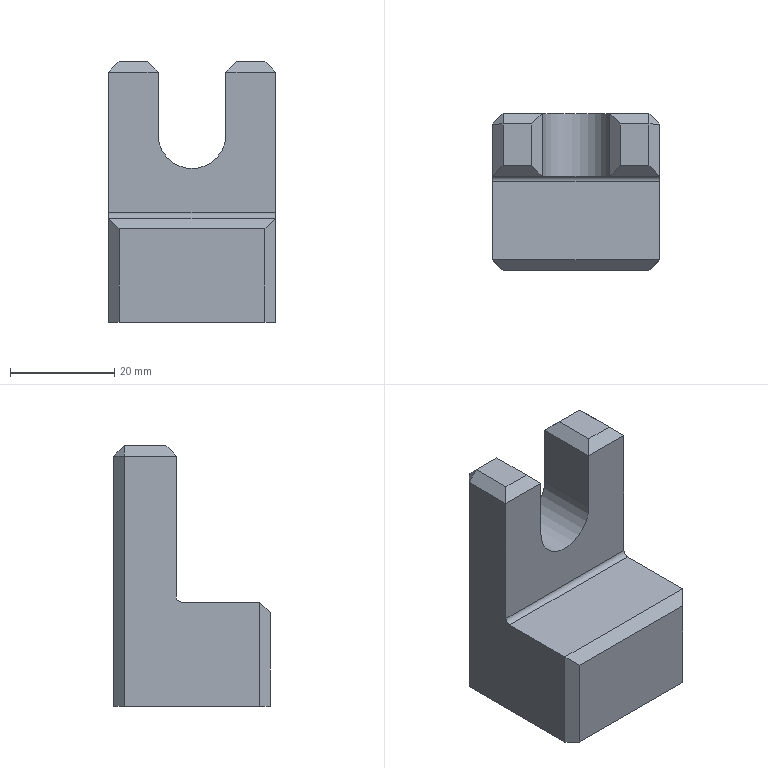Part | NX | features solid 2 | 1 solid | 30 faces | box 32 x 30 x 50 mm | volume 27056 mm3 | plane 26 | cylinder 3 | cone 1 | commonest cylinder face diameters 2 x1 5 x1 13 x1
STEP:
#1=CARTESIAN_POINT('',(8.5,703.,-103.));
#2=VERTEX_POINT('',#1);
#3=CARTESIAN_POINT('',(8.5,695.,-103.));
#4=VERTEX_POINT('',#3);
#5=CARTESIAN_POINT('',(8.5,693.,-103.));
#6=DIRECTION('',(0.,-1.,0.));
#7=VECTOR('',#6,1000.);
#8=LINE('',#5,#7);
#9=EDGE_CURVE('',#2,#4,#8,.T.);
#10=ORIENTED_EDGE('',*,*,#9,.T.);
#11=CARTESIAN_POINT('',(14.,695.,-103.));
#12=VERTEX_POINT('',#11);
#13=CARTESIAN_POINT('',(-16.,695.,-103.));
#14=DIRECTION('',(1.,0.,0.));
#15=VECTOR('',#14,1000.);
#16=LINE('',#13,#15);
#17=EDGE_CURVE('',#4,#12,#16,.T.);
#18=ORIENTED_EDGE('',*,*,#17,.T.);
#19=CARTESIAN_POINT('',(14.,703.,-103.));
#20=VERTEX_POINT('',#19);
#21=CARTESIAN_POINT('',(14.,705.,-103.));
#22=DIRECTION('',(0.,1.,0.));
#23=VECTOR('',#22,1000.);
#24=LINE('',#21,#23);
#25=EDGE_CURVE('',#12,#20,#24,.T.);
#26=ORIENTED_EDGE('',*,*,#25,.T.);
#27=CARTESIAN_POINT('',(6.5,703.,-103.));
#28=DIRECTION('',(-1.,0.,0.));
#29=VECTOR('',#28,1000.);
#30=LINE('',#27,#29);
#31=EDGE_CURVE('',#20,#2,#30,.T.);
#32=ORIENTED_EDGE('',*,*,#31,.T.);
#33=EDGE_LOOP('',(#10,#18,#26,#32));
#34=FACE_BOUND('',#33,.T.);
#35=CARTESIAN_POINT('',(-16.,693.,-103.));
#36=DIRECTION('',(0.,0.,1.));
#37=DIRECTION('',(-1.,0.,0.));
#38=AXIS2_PLACEMENT_3D('',#35,#36,#37);
#39=PLANE('',#38);
#40=ADVANCED_FACE('',(#34),#39,.T.);
#41=CARTESIAN_POINT('',(16.,703.,-153.));
#42=VERTEX_POINT('',#41);
#43=CARTESIAN_POINT('',(16.,703.,-105.));
#44=VERTEX_POINT('',#43);
#45=CARTESIAN_POINT('',(16.,703.,-133.));
#46=DIRECTION('',(0.,0.,1.));
#47=VECTOR('',#46,1000.);
#48=LINE('',#45,#47);
#49=EDGE_CURVE('',#42,#44,#48,.T.);
#50=ORIENTED_EDGE('',*,*,#49,.T.);
#51=CARTESIAN_POINT('',(16.,693.,-105.));
#52=VERTEX_POINT('',#51);
#53=CARTESIAN_POINT('',(16.,693.,-105.));
#54=DIRECTION('',(0.,-1.,0.));
#55=VECTOR('',#54,1000.);
#56=LINE('',#53,#55);
#57=EDGE_CURVE('',#44,#52,#56,.T.);
#58=ORIENTED_EDGE('',*,*,#57,.T.);
#59=CARTESIAN_POINT('',(16.,693.,-132.));
#60=VERTEX_POINT('',#59);
#61=CARTESIAN_POINT('',(16.,693.,-103.));
#62=DIRECTION('',(0.,0.,1.));
#63=VECTOR('',#62,1000.);
#64=LINE('',#61,#63);
#65=EDGE_CURVE('',#60,#52,#64,.T.);
#66=ORIENTED_EDGE('',*,*,#65,.F.);
#67=CARTESIAN_POINT('',(16.,692.,-133.));
#68=VERTEX_POINT('',#67);
#69=CARTESIAN_POINT('',(16.,692.,-132.));
#70=DIRECTION('',(-1.,0.,0.));
#71=DIRECTION('',(0.,0.,-1.));
#72=AXIS2_PLACEMENT_3D('',#69,#70,#71);
#73=CIRCLE('',#72,1.);
#74=EDGE_CURVE('',#60,#68,#73,.T.);
#75=ORIENTED_EDGE('',*,*,#74,.T.);
#76=CARTESIAN_POINT('',(16.,677.,-133.));
#77=VERTEX_POINT('',#76);
#78=CARTESIAN_POINT('',(16.,675.,-133.));
#79=DIRECTION('',(0.,1.,0.));
#80=VECTOR('',#79,1000.);
#81=LINE('',#78,#80);
#82=EDGE_CURVE('',#77,#68,#81,.T.);
#83=ORIENTED_EDGE('',*,*,#82,.F.);
#84=CARTESIAN_POINT('',(16.,677.,-153.));
#85=VERTEX_POINT('',#84);
#86=CARTESIAN_POINT('',(16.,677.,-153.));
#87=DIRECTION('',(0.,0.,-1.));
#88=VECTOR('',#87,1000.);
#89=LINE('',#86,#88);
#90=EDGE_CURVE('',#77,#85,#89,.T.);
#91=ORIENTED_EDGE('',*,*,#90,.T.);
#92=CARTESIAN_POINT('',(16.,675.,-153.));
#93=DIRECTION('',(0.,1.,0.));
#94=VECTOR('',#93,1000.);
#95=LINE('',#92,#94);
#96=EDGE_CURVE('',#85,#42,#95,.T.);
#97=ORIENTED_EDGE('',*,*,#96,.T.);
#98=EDGE_LOOP('',(#50,#58,#66,#75,#83,#91,#97));
#99=FACE_BOUND('',#98,.T.);
#100=CARTESIAN_POINT('',(16.,675.,-133.));
#101=DIRECTION('',(-1.,0.,0.));
#102=DIRECTION('',(0.,0.,-1.));
#103=AXIS2_PLACEMENT_3D('',#100,#101,#102);
#104=PLANE('',#103);
#105=ADVANCED_FACE('',(#99),#104,.F.);
#106=CARTESIAN_POINT('',(0.,705.,-145.5));
#107=VERTEX_POINT('',#106);
#108=CARTESIAN_POINT('',(0.,705.,-143.));
#109=DIRECTION('',(0.,-1.,0.));
#110=DIRECTION('',(0.,0.,-1.));
#111=AXIS2_PLACEMENT_3D('',#108,#109,#110);
#112=CIRCLE('',#111,2.5);
#113=EDGE_CURVE('',#107,#107,#112,.T.);
#114=ORIENTED_EDGE('',*,*,#113,.T.);
#115=EDGE_LOOP('',(#114));
#116=FACE_BOUND('',#115,.T.);
#117=CARTESIAN_POINT('',(6.5,705.,-117.));
#118=VERTEX_POINT('',#117);
#119=CARTESIAN_POINT('',(6.5,705.,-105.));
#120=VERTEX_POINT('',#119);
#121=CARTESIAN_POINT('',(6.5,705.,-103.));
#122=DIRECTION('',(0.,0.,1.));
#123=VECTOR('',#122,1000.);
#124=LINE('',#121,#123);
#125=EDGE_CURVE('',#118,#120,#124,.T.);
#126=ORIENTED_EDGE('',*,*,#125,.T.);
#127=CARTESIAN_POINT('',(14.,705.,-105.));
#128=VERTEX_POINT('',#127);
#129=CARTESIAN_POINT('',(16.,705.,-105.));
#130=DIRECTION('',(1.,0.,0.));
#131=VECTOR('',#130,1000.);
#132=LINE('',#129,#131);
#133=EDGE_CURVE('',#120,#128,#132,.T.);
#134=ORIENTED_EDGE('',*,*,#133,.T.);
#135=CARTESIAN_POINT('',(14.,705.,-153.));
#136=VERTEX_POINT('',#135);
#137=CARTESIAN_POINT('',(14.,705.,-133.));
#138=DIRECTION('',(0.,0.,-1.));
#139=VECTOR('',#138,1000.);
#140=LINE('',#137,#139);
#141=EDGE_CURVE('',#128,#136,#140,.T.);
#142=ORIENTED_EDGE('',*,*,#141,.T.);
#143=CARTESIAN_POINT('',(-14.,705.,-153.));
#144=VERTEX_POINT('',#143);
#145=CARTESIAN_POINT('',(16.,705.,-153.));
#146=DIRECTION('',(-1.,0.,0.));
#147=VECTOR('',#146,1000.);
#148=LINE('',#145,#147);
#149=EDGE_CURVE('',#136,#144,#148,.T.);
#150=ORIENTED_EDGE('',*,*,#149,.T.);
#151=CARTESIAN_POINT('',(-14.,705.,-105.));
#152=VERTEX_POINT('',#151);
#153=CARTESIAN_POINT('',(-14.,705.,-103.));
#154=DIRECTION('',(0.,0.,1.));
#155=VECTOR('',#154,1000.);
#156=LINE('',#153,#155);
#157=EDGE_CURVE('',#144,#152,#156,.T.);
#158=ORIENTED_EDGE('',*,*,#157,.T.);
#159=CARTESIAN_POINT('',(-6.5,705.,-105.));
#160=VERTEX_POINT('',#159);
#161=CARTESIAN_POINT('',(-6.5,705.,-105.));
#162=DIRECTION('',(1.,0.,0.));
#163=VECTOR('',#162,1000.);
#164=LINE('',#161,#163);
#165=EDGE_CURVE('',#152,#160,#164,.T.);
#166=ORIENTED_EDGE('',*,*,#165,.T.);
#167=CARTESIAN_POINT('',(-6.5,705.,-117.));
#168=VERTEX_POINT('',#167);
#169=CARTESIAN_POINT('',(-6.5,705.,-103.));
#170=DIRECTION('',(0.,0.,1.));
#171=VECTOR('',#170,1000.);
#172=LINE('',#169,#171);
#173=EDGE_CURVE('',#168,#160,#172,.T.);
#174=ORIENTED_EDGE('',*,*,#173,.F.);
#175=CARTESIAN_POINT('',(0.,705.,-117.));
#176=DIRECTION('',(0.,1.,0.));
#177=DIRECTION('',(0.,0.,1.));
#178=AXIS2_PLACEMENT_3D('',#175,#176,#177);
#179=CIRCLE('',#178,6.5);
#180=EDGE_CURVE('',#118,#168,#179,.T.);
#181=ORIENTED_EDGE('',*,*,#180,.F.);
#182=EDGE_LOOP('',(#126,#134,#142,#150,#158,#166,#174,#181));
#183=FACE_BOUND('',#182,.T.);
#184=CARTESIAN_POINT('',(16.,705.,-133.));
#185=DIRECTION('',(0.,-1.,0.));
#186=DIRECTION('',(0.,0.,-1.));
#187=AXIS2_PLACEMENT_3D('',#184,#185,#186);
#188=PLANE('',#187);
#189=ADVANCED_FACE('',(#116,#183),#188,.F.);
#190=CARTESIAN_POINT('',(-16.,677.,-133.));
#191=VERTEX_POINT('',#190);
#192=CARTESIAN_POINT('',(-16.,692.,-133.));
#193=VERTEX_POINT('',#192);
#194=CARTESIAN_POINT('',(-16.,675.,-133.));
#195=DIRECTION('',(0.,1.,0.));
#196=VECTOR('',#195,1000.);
#197=LINE('',#194,#196);
#198=EDGE_CURVE('',#191,#193,#197,.T.);
#199=ORIENTED_EDGE('',*,*,#198,.T.);
#200=CARTESIAN_POINT('',(-16.,693.,-132.));
#201=VERTEX_POINT('',#200);
#202=CARTESIAN_POINT('',(-16.,692.,-132.));
#203=DIRECTION('',(-1.,0.,0.));
#204=DIRECTION('',(0.,0.,-1.));
#205=AXIS2_PLACEMENT_3D('',#202,#203,#204);
#206=CIRCLE('',#205,1.);
#207=EDGE_CURVE('',#193,#201,#206,.F.);
#208=ORIENTED_EDGE('',*,*,#207,.T.);
#209=CARTESIAN_POINT('',(-16.,693.,-105.));
#210=VERTEX_POINT('',#209);
#211=CARTESIAN_POINT('',(-16.,693.,-103.));
#212=DIRECTION('',(0.,0.,1.));
#213=VECTOR('',#212,1000.);
#214=LINE('',#211,#213);
#215=EDGE_CURVE('',#201,#210,#214,.T.);
#216=ORIENTED_EDGE('',*,*,#215,.T.);
#217=CARTESIAN_POINT('',(-16.,703.,-105.));
#218=VERTEX_POINT('',#217);
#219=CARTESIAN_POINT('',(-16.,675.,-105.));
#220=DIRECTION('',(0.,1.,0.));
#221=VECTOR('',#220,1000.);
#222=LINE('',#219,#221);
#223=EDGE_CURVE('',#210,#218,#222,.T.);
#224=ORIENTED_EDGE('',*,*,#223,.T.);
#225=CARTESIAN_POINT('',(-16.,703.,-153.));
#226=VERTEX_POINT('',#225);
#227=CARTESIAN_POINT('',(-16.,703.,-153.));
#228=DIRECTION('',(0.,0.,-1.));
#229=VECTOR('',#228,1000.);
#230=LINE('',#227,#229);
#231=EDGE_CURVE('',#218,#226,#230,.T.);
#232=ORIENTED_EDGE('',*,*,#231,.T.);
#233=CARTESIAN_POINT('',(-16.,677.,-153.));
#234=VERTEX_POINT('',#233);
#235=CARTESIAN_POINT('',(-16.,675.,-153.));
#236=DIRECTION('',(0.,1.,0.));
#237=VECTOR('',#236,1000.);
#238=LINE('',#235,#237);
#239=EDGE_CURVE('',#234,#226,#238,.T.);
#240=ORIENTED_EDGE('',*,*,#239,.F.);
#241=CARTESIAN_POINT('',(-16.,677.,-133.));
#242=DIRECTION('',(0.,0.,1.));
#243=VECTOR('',#242,1000.);
#244=LINE('',#241,#243);
#245=EDGE_CURVE('',#234,#191,#244,.T.);
#246=ORIENTED_EDGE('',*,*,#245,.T.);
#247=EDGE_LOOP('',(#199,#208,#216,#224,#232,#240,#246));
#248=FACE_BOUND('',#247,.T.);
#249=CARTESIAN_POINT('',(-16.,675.,-133.));
#250=DIRECTION('',(-1.,0.,0.));
#251=DIRECTION('',(0.,0.,-1.));
#252=AXIS2_PLACEMENT_3D('',#249,#250,#251);
#253=PLANE('',#252);
#254=ADVANCED_FACE('',(#248),#253,.T.);
#255=CARTESIAN_POINT('',(14.,675.,-153.));
#256=VERTEX_POINT('',#255);
#257=CARTESIAN_POINT('',(-14.,675.,-153.));
#258=VERTEX_POINT('',#257);
#259=CARTESIAN_POINT('',(16.,675.,-153.));
#260=DIRECTION('',(-1.,0.,0.));
#261=VECTOR('',#260,1000.);
#262=LINE('',#259,#261);
#263=EDGE_CURVE('',#256,#258,#262,.T.);
#264=ORIENTED_EDGE('',*,*,#263,.F.);
#265=CARTESIAN_POINT('',(14.,675.,-135.));
#266=VERTEX_POINT('',#265);
#267=CARTESIAN_POINT('',(14.,675.,-133.));
#268=DIRECTION('',(0.,0.,1.));
#269=VECTOR('',#268,1000.);
#270=LINE('',#267,#269);
#271=EDGE_CURVE('',#256,#266,#270,.T.);
#272=ORIENTED_EDGE('',*,*,#271,.T.);
#273=CARTESIAN_POINT('',(-14.,675.,-135.));
#274=VERTEX_POINT('',#273);
#275=CARTESIAN_POINT('',(16.,675.,-135.));
#276=DIRECTION('',(-1.,0.,0.));
#277=VECTOR('',#276,1000.);
#278=LINE('',#275,#277);
#279=EDGE_CURVE('',#266,#274,#278,.T.);
#280=ORIENTED_EDGE('',*,*,#279,.T.);
#281=CARTESIAN_POINT('',(-14.,675.,-133.));
#282=DIRECTION('',(0.,0.,-1.));
#283=VECTOR('',#282,1000.);
#284=LINE('',#281,#283);
#285=EDGE_CURVE('',#274,#258,#284,.T.);
#286=ORIENTED_EDGE('',*,*,#285,.T.);
#287=EDGE_LOOP('',(#264,#272,#280,#286));
#288=FACE_BOUND('',#287,.T.);
#289=CARTESIAN_POINT('',(16.,675.,-133.));
#290=DIRECTION('',(0.,-1.,0.));
#291=DIRECTION('',(0.,0.,-1.));
#292=AXIS2_PLACEMENT_3D('',#289,#290,#291);
#293=PLANE('',#292);
#294=ADVANCED_FACE('',(#288),#293,.T.);
#295=ORIENTED_EDGE('',*,*,#82,.T.);
#296=CARTESIAN_POINT('',(-16.,692.,-133.));
#297=DIRECTION('',(1.,0.,0.));
#298=VECTOR('',#297,1000.);
#299=LINE('',#296,#298);
#300=EDGE_CURVE('',#68,#193,#299,.F.);
#301=ORIENTED_EDGE('',*,*,#300,.T.);
#302=ORIENTED_EDGE('',*,*,#198,.F.);
#303=CARTESIAN_POINT('',(16.,677.,-133.));
#304=DIRECTION('',(1.,0.,0.));
#305=VECTOR('',#304,1000.);
#306=LINE('',#303,#305);
#307=EDGE_CURVE('',#191,#77,#306,.T.);
#308=ORIENTED_EDGE('',*,*,#307,.T.);
#309=EDGE_LOOP('',(#295,#301,#302,#308));
#310=FACE_BOUND('',#309,.T.);
#311=CARTESIAN_POINT('',(16.,705.,-133.));
#312=DIRECTION('',(0.,0.,1.));
#313=DIRECTION('',(-1.,0.,0.));
#314=AXIS2_PLACEMENT_3D('',#311,#312,#313);
#315=PLANE('',#314);
#316=ADVANCED_FACE('',(#310),#315,.T.);
#317=ORIENTED_EDGE('',*,*,#149,.F.);
#318=CARTESIAN_POINT('',(14.,705.,-153.));
#319=DIRECTION('',(-0.7071,0.7071,0.));
#320=VECTOR('',#319,1000.);
#321=LINE('',#318,#320);
#322=EDGE_CURVE('',#136,#42,#321,.F.);
#323=ORIENTED_EDGE('',*,*,#322,.T.);
#324=ORIENTED_EDGE('',*,*,#96,.F.);
#325=CARTESIAN_POINT('',(16.,677.,-153.));
#326=DIRECTION('',(-0.7071,-0.7071,0.));
#327=VECTOR('',#326,1000.);
#328=LINE('',#325,#327);
#329=EDGE_CURVE('',#85,#256,#328,.T.);
#330=ORIENTED_EDGE('',*,*,#329,.T.);
#331=ORIENTED_EDGE('',*,*,#263,.T.);
#332=CARTESIAN_POINT('',(-14.,675.,-153.));
#333=DIRECTION('',(0.7071,-0.7071,0.));
#334=VECTOR('',#333,1000.);
#335=LINE('',#332,#334);
#336=EDGE_CURVE('',#258,#234,#335,.F.);
#337=ORIENTED_EDGE('',*,*,#336,.T.);
#338=ORIENTED_EDGE('',*,*,#239,.T.);
#339=CARTESIAN_POINT('',(-16.,703.,-153.));
#340=DIRECTION('',(0.7071,0.7071,0.));
#341=VECTOR('',#340,1000.);
#342=LINE('',#339,#341);
#343=EDGE_CURVE('',#226,#144,#342,.T.);
#344=ORIENTED_EDGE('',*,*,#343,.T.);
#345=EDGE_LOOP('',(#317,#323,#324,#330,#331,#337,#338,#344));
#346=FACE_BOUND('',#345,.T.);
#347=CARTESIAN_POINT('',(16.,705.,-153.));
#348=DIRECTION('',(0.,0.,1.));
#349=DIRECTION('',(-1.,0.,0.));
#350=AXIS2_PLACEMENT_3D('',#347,#348,#349);
#351=PLANE('',#350);
#352=ADVANCED_FACE('',(#346),#351,.F.);
#353=ORIENTED_EDGE('',*,*,#215,.F.);
#354=CARTESIAN_POINT('',(16.,693.,-132.));
#355=DIRECTION('',(1.,0.,0.));
#356=VECTOR('',#355,1000.);
#357=LINE('',#354,#356);
#358=EDGE_CURVE('',#201,#60,#357,.T.);
#359=ORIENTED_EDGE('',*,*,#358,.T.);
#360=ORIENTED_EDGE('',*,*,#65,.T.);
#361=CARTESIAN_POINT('',(6.5,693.,-105.));
#362=VERTEX_POINT('',#361);
#363=CARTESIAN_POINT('',(16.,693.,-105.));
#364=DIRECTION('',(-1.,0.,0.));
#365=VECTOR('',#364,1000.);
#366=LINE('',#363,#365);
#367=EDGE_CURVE('',#52,#362,#366,.T.);
#368=ORIENTED_EDGE('',*,*,#367,.T.);
#369=CARTESIAN_POINT('',(6.5,693.,-117.));
#370=VERTEX_POINT('',#369);
#371=CARTESIAN_POINT('',(6.5,693.,-133.));
#372=DIRECTION('',(0.,0.,1.));
#373=VECTOR('',#372,1000.);
#374=LINE('',#371,#373);
#375=EDGE_CURVE('',#370,#362,#374,.T.);
#376=ORIENTED_EDGE('',*,*,#375,.F.);
#377=CARTESIAN_POINT('',(-6.5,693.,-117.));
#378=VERTEX_POINT('',#377);
#379=CARTESIAN_POINT('',(0.,693.,-117.));
#380=DIRECTION('',(0.,-1.,0.));
#381=DIRECTION('',(0.,0.,-1.));
#382=AXIS2_PLACEMENT_3D('',#379,#380,#381);
#383=CIRCLE('',#382,6.5);
#384=EDGE_CURVE('',#378,#370,#383,.T.);
#385=ORIENTED_EDGE('',*,*,#384,.F.);
#386=CARTESIAN_POINT('',(-6.5,693.,-105.));
#387=VERTEX_POINT('',#386);
#388=CARTESIAN_POINT('',(-6.5,693.,-133.));
#389=DIRECTION('',(0.,0.,-1.));
#390=VECTOR('',#389,1000.);
#391=LINE('',#388,#390);
#392=EDGE_CURVE('',#387,#378,#391,.T.);
#393=ORIENTED_EDGE('',*,*,#392,.F.);
#394=CARTESIAN_POINT('',(16.,693.,-105.));
#395=DIRECTION('',(-1.,0.,0.));
#396=VECTOR('',#395,1000.);
#397=LINE('',#394,#396);
#398=EDGE_CURVE('',#387,#210,#397,.T.);
#399=ORIENTED_EDGE('',*,*,#398,.T.);
#400=EDGE_LOOP('',(#353,#359,#360,#368,#376,#385,#393,#399));
#401=FACE_BOUND('',#400,.T.);
#402=CARTESIAN_POINT('',(16.,693.,-133.));
#403=DIRECTION('',(0.,-1.,0.));
#404=DIRECTION('',(0.,0.,-1.));
#405=AXIS2_PLACEMENT_3D('',#402,#403,#404);
#406=PLANE('',#405);
#407=ADVANCED_FACE('',(#401),#406,.T.);
#408=CARTESIAN_POINT('',(-14.,703.,-103.));
#409=VERTEX_POINT('',#408);
#410=CARTESIAN_POINT('',(-14.,695.,-103.));
#411=VERTEX_POINT('',#410);
#412=CARTESIAN_POINT('',(-14.,693.,-103.));
#413=DIRECTION('',(0.,-1.,0.));
#414=VECTOR('',#413,1000.);
#415=LINE('',#412,#414);
#416=EDGE_CURVE('',#409,#411,#415,.T.);
#417=ORIENTED_EDGE('',*,*,#416,.T.);
#418=CARTESIAN_POINT('',(-8.5,695.,-103.));
#419=VERTEX_POINT('',#418);
#420=CARTESIAN_POINT('',(-16.,695.,-103.));
#421=DIRECTION('',(1.,0.,0.));
#422=VECTOR('',#421,1000.);
#423=LINE('',#420,#422);
#424=EDGE_CURVE('',#411,#419,#423,.T.);
#425=ORIENTED_EDGE('',*,*,#424,.T.);
#426=CARTESIAN_POINT('',(-8.5,703.,-103.));
#427=VERTEX_POINT('',#426);
#428=CARTESIAN_POINT('',(-8.5,705.,-103.));
#429=DIRECTION('',(0.,1.,0.));
#430=VECTOR('',#429,1000.);
#431=LINE('',#428,#430);
#432=EDGE_CURVE('',#419,#427,#431,.T.);
#433=ORIENTED_EDGE('',*,*,#432,.T.);
#434=CARTESIAN_POINT('',(-16.,703.,-103.));
#435=DIRECTION('',(-1.,0.,0.));
#436=VECTOR('',#435,1000.);
#437=LINE('',#434,#436);
#438=EDGE_CURVE('',#427,#409,#437,.T.);
#439=ORIENTED_EDGE('',*,*,#438,.T.);
#440=EDGE_LOOP('',(#417,#425,#433,#439));
#441=FACE_BOUND('',#440,.T.);
#442=CARTESIAN_POINT('',(-16.,693.,-103.));
#443=DIRECTION('',(0.,0.,1.));
#444=DIRECTION('',(-1.,0.,0.));
#445=AXIS2_PLACEMENT_3D('',#442,#443,#444);
#446=PLANE('',#445);
#447=ADVANCED_FACE('',(#441),#446,.T.);
#448=ORIENTED_EDGE('',*,*,#375,.T.);
#449=CARTESIAN_POINT('',(6.5,705.,-105.));
#450=DIRECTION('',(0.,1.,0.));
#451=VECTOR('',#450,1000.);
#452=LINE('',#449,#451);
#453=EDGE_CURVE('',#362,#120,#452,.T.);
#454=ORIENTED_EDGE('',*,*,#453,.T.);
#455=ORIENTED_EDGE('',*,*,#125,.F.);
#456=CARTESIAN_POINT('',(6.5,705.,-117.));
#457=DIRECTION('',(0.,1.,0.));
#458=VECTOR('',#457,1000.);
#459=LINE('',#456,#458);
#460=EDGE_CURVE('',#370,#118,#459,.T.);
#461=ORIENTED_EDGE('',*,*,#460,.F.);
#462=EDGE_LOOP('',(#448,#454,#455,#461));
#463=FACE_BOUND('',#462,.T.);
#464=CARTESIAN_POINT('',(6.5,705.,-103.));
#465=DIRECTION('',(1.,0.,0.));
#466=DIRECTION('',(0.,0.,1.));
#467=AXIS2_PLACEMENT_3D('',#464,#465,#466);
#468=PLANE('',#467);
#469=ADVANCED_FACE('',(#463),#468,.F.);
#470=ORIENTED_EDGE('',*,*,#384,.T.);
#471=ORIENTED_EDGE('',*,*,#460,.T.);
#472=ORIENTED_EDGE('',*,*,#180,.T.);
#473=CARTESIAN_POINT('',(-6.5,705.,-117.));
#474=DIRECTION('',(0.,1.,0.));
#475=VECTOR('',#474,1000.);
#476=LINE('',#473,#475);
#477=EDGE_CURVE('',#378,#168,#476,.T.);
#478=ORIENTED_EDGE('',*,*,#477,.F.);
#479=EDGE_LOOP('',(#470,#471,#472,#478));
#480=FACE_BOUND('',#479,.T.);
#481=CARTESIAN_POINT('',(0.,705.,-117.));
#482=DIRECTION('',(0.,1.,0.));
#483=DIRECTION('',(0.,0.,1.));
#484=AXIS2_PLACEMENT_3D('',#481,#482,#483);
#485=CYLINDRICAL_SURFACE('',#484,6.5);
#486=ADVANCED_FACE('',(#480),#485,.F.);
#487=ORIENTED_EDGE('',*,*,#173,.T.);
#488=CARTESIAN_POINT('',(-6.5,693.,-105.));
#489=DIRECTION('',(0.,-1.,0.));
#490=VECTOR('',#489,1000.);
#491=LINE('',#488,#490);
#492=EDGE_CURVE('',#160,#387,#491,.T.);
#493=ORIENTED_EDGE('',*,*,#492,.T.);
#494=ORIENTED_EDGE('',*,*,#392,.T.);
#495=ORIENTED_EDGE('',*,*,#477,.T.);
#496=EDGE_LOOP('',(#487,#493,#494,#495));
#497=FACE_BOUND('',#496,.T.);
#498=CARTESIAN_POINT('',(-6.5,705.,-103.));
#499=DIRECTION('',(-1.,0.,0.));
#500=DIRECTION('',(0.,0.,-1.));
#501=AXIS2_PLACEMENT_3D('',#498,#499,#500);
#502=PLANE('',#501);
#503=ADVANCED_FACE('',(#497),#502,.F.);
#504=CARTESIAN_POINT('',(-16.,703.,-105.));
#505=DIRECTION('',(-0.7071,-0.7071,0.));
#506=VECTOR('',#505,1000.);
#507=LINE('',#504,#506);
#508=EDGE_CURVE('',#152,#218,#507,.T.);
#509=ORIENTED_EDGE('',*,*,#508,.F.);
#510=ORIENTED_EDGE('',*,*,#157,.F.);
#511=ORIENTED_EDGE('',*,*,#343,.F.);
#512=ORIENTED_EDGE('',*,*,#231,.F.);
#513=EDGE_LOOP('',(#509,#510,#511,#512));
#514=FACE_BOUND('',#513,.T.);
#515=CARTESIAN_POINT('',(-16.,703.,-133.));
#516=DIRECTION('',(-0.7071,0.7071,0.));
#517=DIRECTION('',(-0.7071,-0.7071,0.));
#518=AXIS2_PLACEMENT_3D('',#515,#516,#517);
#519=PLANE('',#518);
#520=ADVANCED_FACE('',(#514),#519,.T.);
#521=CARTESIAN_POINT('',(-16.,703.,-105.));
#522=DIRECTION('',(-0.7071,0.,-0.7071));
#523=VECTOR('',#522,1000.);
#524=LINE('',#521,#523);
#525=EDGE_CURVE('',#409,#218,#524,.T.);
#526=ORIENTED_EDGE('',*,*,#525,.F.);
#527=CARTESIAN_POINT('',(-14.,704.,-104.));
#528=DIRECTION('',(0.,0.7071,-0.7071));
#529=VECTOR('',#528,1000.);
#530=LINE('',#527,#529);
#531=EDGE_CURVE('',#152,#409,#530,.F.);
#532=ORIENTED_EDGE('',*,*,#531,.F.);
#533=ORIENTED_EDGE('',*,*,#508,.T.);
#534=EDGE_LOOP('',(#526,#532,#533));
#535=FACE_BOUND('',#534,.T.);
#536=CARTESIAN_POINT('',(-16.,703.,-105.));
#537=DIRECTION('',(-0.5774,0.5774,0.5774));
#538=DIRECTION('',(-0.7071,-0.7071,0.));
#539=AXIS2_PLACEMENT_3D('',#536,#537,#538);
#540=PLANE('',#539);
#541=ADVANCED_FACE('',(#535),#540,.T.);
#542=ORIENTED_EDGE('',*,*,#531,.T.);
#543=ORIENTED_EDGE('',*,*,#438,.F.);
#544=CARTESIAN_POINT('',(-6.5,705.,-105.));
#545=DIRECTION('',(-0.5774,-0.5774,0.5774));
#546=VECTOR('',#545,1000.);
#547=LINE('',#544,#546);
#548=EDGE_CURVE('',#160,#427,#547,.T.);
#549=ORIENTED_EDGE('',*,*,#548,.F.);
#550=ORIENTED_EDGE('',*,*,#165,.F.);
#551=EDGE_LOOP('',(#542,#543,#549,#550));
#552=FACE_BOUND('',#551,.T.);
#553=CARTESIAN_POINT('',(16.,705.,-105.));
#554=DIRECTION('',(0.,0.7071,0.7071));
#555=DIRECTION('',(0.,-0.7071,0.7071));
#556=AXIS2_PLACEMENT_3D('',#553,#554,#555);
#557=PLANE('',#556);
#558=ADVANCED_FACE('',(#552),#557,.T.);
#559=ORIENTED_EDGE('',*,*,#525,.T.);
#560=ORIENTED_EDGE('',*,*,#223,.F.);
#561=CARTESIAN_POINT('',(-22.,687.,-111.));
#562=DIRECTION('',(0.5774,0.5774,0.5774));
#563=VECTOR('',#562,1000.);
#564=LINE('',#561,#563);
#565=EDGE_CURVE('',#411,#210,#564,.F.);
#566=ORIENTED_EDGE('',*,*,#565,.F.);
#567=ORIENTED_EDGE('',*,*,#416,.F.);
#568=EDGE_LOOP('',(#559,#560,#566,#567));
#569=FACE_BOUND('',#568,.T.);
#570=CARTESIAN_POINT('',(-16.,675.,-105.));
#571=DIRECTION('',(0.7071,0.,-0.7071));
#572=DIRECTION('',(0.7071,0.,0.7071));
#573=AXIS2_PLACEMENT_3D('',#570,#571,#572);
#574=PLANE('',#573);
#575=ADVANCED_FACE('',(#569),#574,.F.);
#576=ORIENTED_EDGE('',*,*,#548,.T.);
#577=ORIENTED_EDGE('',*,*,#432,.F.);
#578=CARTESIAN_POINT('',(-10.5,697.,-101.));
#579=DIRECTION('',(-0.5774,0.5774,0.5774));
#580=VECTOR('',#579,1000.);
#581=LINE('',#578,#580);
#582=EDGE_CURVE('',#387,#419,#581,.T.);
#583=ORIENTED_EDGE('',*,*,#582,.F.);
#584=ORIENTED_EDGE('',*,*,#492,.F.);
#585=EDGE_LOOP('',(#576,#577,#583,#584));
#586=FACE_BOUND('',#585,.T.);
#587=CARTESIAN_POINT('',(-6.5,705.,-105.));
#588=DIRECTION('',(0.7071,0.,0.7071));
#589=DIRECTION('',(-0.7071,0.,0.7071));
#590=AXIS2_PLACEMENT_3D('',#587,#588,#589);
#591=PLANE('',#590);
#592=ADVANCED_FACE('',(#586),#591,.T.);
#593=ORIENTED_EDGE('',*,*,#565,.T.);
#594=ORIENTED_EDGE('',*,*,#398,.F.);
#595=ORIENTED_EDGE('',*,*,#582,.T.);
#596=ORIENTED_EDGE('',*,*,#424,.F.);
#597=EDGE_LOOP('',(#593,#594,#595,#596));
#598=FACE_BOUND('',#597,.T.);
#599=CARTESIAN_POINT('',(-16.,695.,-103.));
#600=DIRECTION('',(0.,0.7071,-0.7071));
#601=DIRECTION('',(0.,0.7071,0.7071));
#602=AXIS2_PLACEMENT_3D('',#599,#600,#601);
#603=PLANE('',#602);
#604=ADVANCED_FACE('',(#598),#603,.F.);
#605=ORIENTED_EDGE('',*,*,#322,.F.);
#606=ORIENTED_EDGE('',*,*,#141,.F.);
#607=CARTESIAN_POINT('',(14.,705.,-105.));
#608=DIRECTION('',(0.7071,-0.7071,0.));
#609=VECTOR('',#608,1000.);
#610=LINE('',#607,#609);
#611=EDGE_CURVE('',#44,#128,#610,.F.);
#612=ORIENTED_EDGE('',*,*,#611,.F.);
#613=ORIENTED_EDGE('',*,*,#49,.F.);
#614=EDGE_LOOP('',(#605,#606,#612,#613));
#615=FACE_BOUND('',#614,.T.);
#616=CARTESIAN_POINT('',(14.,705.,-133.));
#617=DIRECTION('',(-0.7071,-0.7071,0.));
#618=DIRECTION('',(0.7071,-0.7071,0.));
#619=AXIS2_PLACEMENT_3D('',#616,#617,#618);
#620=PLANE('',#619);
#621=ADVANCED_FACE('',(#615),#620,.F.);
#622=CARTESIAN_POINT('',(14.,705.,-105.));
#623=DIRECTION('',(0.,-0.7071,0.7071));
#624=VECTOR('',#623,1000.);
#625=LINE('',#622,#624);
#626=EDGE_CURVE('',#128,#20,#625,.T.);
#627=ORIENTED_EDGE('',*,*,#626,.F.);
#628=ORIENTED_EDGE('',*,*,#133,.F.);
#629=CARTESIAN_POINT('',(9.667,701.833,-101.833));
#630=DIRECTION('',(0.5774,-0.5774,0.5774));
#631=VECTOR('',#630,1000.);
#632=LINE('',#629,#631);
#633=EDGE_CURVE('',#2,#120,#632,.F.);
#634=ORIENTED_EDGE('',*,*,#633,.F.);
#635=ORIENTED_EDGE('',*,*,#31,.F.);
#636=EDGE_LOOP('',(#627,#628,#634,#635));
#637=FACE_BOUND('',#636,.T.);
#638=CARTESIAN_POINT('',(16.,705.,-105.));
#639=DIRECTION('',(0.,0.7071,0.7071));
#640=DIRECTION('',(0.,-0.7071,0.7071));
#641=AXIS2_PLACEMENT_3D('',#638,#639,#640);
#642=PLANE('',#641);
#643=ADVANCED_FACE('',(#637),#642,.T.);
#644=ORIENTED_EDGE('',*,*,#611,.T.);
#645=ORIENTED_EDGE('',*,*,#626,.T.);
#646=CARTESIAN_POINT('',(15.,703.,-104.));
#647=DIRECTION('',(0.7071,0.,-0.7071));
#648=VECTOR('',#647,1000.);
#649=LINE('',#646,#648);
#650=EDGE_CURVE('',#44,#20,#649,.F.);
#651=ORIENTED_EDGE('',*,*,#650,.F.);
#652=EDGE_LOOP('',(#644,#645,#651));
#653=FACE_BOUND('',#652,.T.);
#654=CARTESIAN_POINT('',(14.,705.,-105.));
#655=DIRECTION('',(0.5774,0.5774,0.5774));
#656=DIRECTION('',(0.,-0.7071,0.7071));
#657=AXIS2_PLACEMENT_3D('',#654,#655,#656);
#658=PLANE('',#657);
#659=ADVANCED_FACE('',(#653),#658,.T.);
#660=ORIENTED_EDGE('',*,*,#633,.T.);
#661=ORIENTED_EDGE('',*,*,#453,.F.);
#662=CARTESIAN_POINT('',(10.5,697.,-101.));
#663=DIRECTION('',(-0.5774,-0.5774,-0.5774));
#664=VECTOR('',#663,1000.);
#665=LINE('',#662,#664);
#666=EDGE_CURVE('',#4,#362,#665,.T.);
#667=ORIENTED_EDGE('',*,*,#666,.F.);
#668=ORIENTED_EDGE('',*,*,#9,.F.);
#669=EDGE_LOOP('',(#660,#661,#667,#668));
#670=FACE_BOUND('',#669,.T.);
#671=CARTESIAN_POINT('',(6.5,705.,-105.));
#672=DIRECTION('',(-0.7071,0.,0.7071));
#673=DIRECTION('',(-0.7071,0.,-0.7071));
#674=AXIS2_PLACEMENT_3D('',#671,#672,#673);
#675=PLANE('',#674);
#676=ADVANCED_FACE('',(#670),#675,.T.);
#677=ORIENTED_EDGE('',*,*,#650,.T.);
#678=ORIENTED_EDGE('',*,*,#25,.F.);
#679=CARTESIAN_POINT('',(14.667,694.333,-103.667));
#680=DIRECTION('',(-0.5774,0.5774,0.5774));
#681=VECTOR('',#680,1000.);
#682=LINE('',#679,#681);
#683=EDGE_CURVE('',#52,#12,#682,.T.);
#684=ORIENTED_EDGE('',*,*,#683,.F.);
#685=ORIENTED_EDGE('',*,*,#57,.F.);
#686=EDGE_LOOP('',(#677,#678,#684,#685));
#687=FACE_BOUND('',#686,.T.);
#688=CARTESIAN_POINT('',(14.,693.,-103.));
#689=DIRECTION('',(0.7071,0.,0.7071));
#690=DIRECTION('',(-0.7071,0.,0.7071));
#691=AXIS2_PLACEMENT_3D('',#688,#689,#690);
#692=PLANE('',#691);
#693=ADVANCED_FACE('',(#687),#692,.T.);
#694=ORIENTED_EDGE('',*,*,#666,.T.);
#695=ORIENTED_EDGE('',*,*,#367,.F.);
#696=ORIENTED_EDGE('',*,*,#683,.T.);
#697=ORIENTED_EDGE('',*,*,#17,.F.);
#698=EDGE_LOOP('',(#694,#695,#696,#697));
#699=FACE_BOUND('',#698,.T.);
#700=CARTESIAN_POINT('',(-16.,695.,-103.));
#701=DIRECTION('',(0.,0.7071,-0.7071));
#702=DIRECTION('',(0.,0.7071,0.7071));
#703=AXIS2_PLACEMENT_3D('',#700,#701,#702);
#704=PLANE('',#703);
#705=ADVANCED_FACE('',(#699),#704,.F.);
#706=ORIENTED_EDGE('',*,*,#329,.F.);
#707=ORIENTED_EDGE('',*,*,#90,.F.);
#708=CARTESIAN_POINT('',(16.,677.,-133.));
#709=DIRECTION('',(0.5774,0.5774,0.5774));
#710=VECTOR('',#709,1000.);
#711=LINE('',#708,#710);
#712=EDGE_CURVE('',#266,#77,#711,.T.);
#713=ORIENTED_EDGE('',*,*,#712,.F.);
#714=ORIENTED_EDGE('',*,*,#271,.F.);
#715=EDGE_LOOP('',(#706,#707,#713,#714));
#716=FACE_BOUND('',#715,.T.);
#717=CARTESIAN_POINT('',(16.,677.,-133.));
#718=DIRECTION('',(0.7071,-0.7071,0.));
#719=DIRECTION('',(0.7071,0.7071,0.));
#720=AXIS2_PLACEMENT_3D('',#717,#718,#719);
#721=PLANE('',#720);
#722=ADVANCED_FACE('',(#716),#721,.T.);
#723=ORIENTED_EDGE('',*,*,#336,.F.);
#724=ORIENTED_EDGE('',*,*,#285,.F.);
#725=CARTESIAN_POINT('',(-14.667,675.667,-134.333));
#726=DIRECTION('',(-0.5774,0.5774,0.5774));
#727=VECTOR('',#726,1000.);
#728=LINE('',#725,#727);
#729=EDGE_CURVE('',#191,#274,#728,.F.);
#730=ORIENTED_EDGE('',*,*,#729,.F.);
#731=ORIENTED_EDGE('',*,*,#245,.F.);
#732=EDGE_LOOP('',(#723,#724,#730,#731));
#733=FACE_BOUND('',#732,.T.);
#734=CARTESIAN_POINT('',(-14.,675.,-133.));
#735=DIRECTION('',(0.7071,0.7071,0.));
#736=DIRECTION('',(-0.7071,0.7071,0.));
#737=AXIS2_PLACEMENT_3D('',#734,#735,#736);
#738=PLANE('',#737);
#739=ADVANCED_FACE('',(#733),#738,.F.);
#740=ORIENTED_EDGE('',*,*,#712,.T.);
#741=ORIENTED_EDGE('',*,*,#307,.F.);
#742=ORIENTED_EDGE('',*,*,#729,.T.);
#743=ORIENTED_EDGE('',*,*,#279,.F.);
#744=EDGE_LOOP('',(#740,#741,#742,#743));
#745=FACE_BOUND('',#744,.T.);
#746=CARTESIAN_POINT('',(16.,675.,-135.));
#747=DIRECTION('',(0.,0.7071,-0.7071));
#748=DIRECTION('',(0.,0.7071,0.7071));
#749=AXIS2_PLACEMENT_3D('',#746,#747,#748);
#750=PLANE('',#749);
#751=ADVANCED_FACE('',(#745),#750,.F.);
#752=ORIENTED_EDGE('',*,*,#207,.F.);
#753=ORIENTED_EDGE('',*,*,#300,.F.);
#754=ORIENTED_EDGE('',*,*,#74,.F.);
#755=ORIENTED_EDGE('',*,*,#358,.F.);
#756=EDGE_LOOP('',(#752,#753,#754,#755));
#757=FACE_BOUND('',#756,.T.);
#758=CARTESIAN_POINT('',(16.,692.,-132.));
#759=DIRECTION('',(-1.,0.,0.));
#760=DIRECTION('',(0.,0.,-1.));
#761=AXIS2_PLACEMENT_3D('',#758,#759,#760);
#762=CYLINDRICAL_SURFACE('',#761,1.);
#763=ADVANCED_FACE('',(#757),#762,.F.);
#764=CARTESIAN_POINT('',(0.,695.,-145.5));
#765=VERTEX_POINT('',#764);
#766=CARTESIAN_POINT('',(0.,695.,-143.));
#767=DIRECTION('',(0.,-1.,0.));
#768=DIRECTION('',(0.,0.,-1.));
#769=AXIS2_PLACEMENT_3D('',#766,#767,#768);
#770=CIRCLE('',#769,2.5);
#771=EDGE_CURVE('',#765,#765,#770,.T.);
#772=ORIENTED_EDGE('',*,*,#771,.F.);
#773=EDGE_LOOP('',(#772));
#774=FACE_BOUND('',#773,.T.);
#775=CARTESIAN_POINT('',(0.,693.498,-143.));
#776=VERTEX_POINT('',#775);
#777=VERTEX_LOOP('',#776);
#778=FACE_BOUND('',#777,.T.);
#779=CARTESIAN_POINT('',(0.,695.,-143.));
#780=DIRECTION('',(0.,1.,0.));
#781=DIRECTION('',(0.,0.,1.));
#782=AXIS2_PLACEMENT_3D('',#779,#780,#781);
#783=CONICAL_SURFACE('',#782,2.5,1.03);
#784=ADVANCED_FACE('',(#774,#778),#783,.F.);
#785=ORIENTED_EDGE('',*,*,#771,.T.);
#786=EDGE_LOOP('',(#785));
#787=FACE_BOUND('',#786,.T.);
#788=ORIENTED_EDGE('',*,*,#113,.F.);
#789=EDGE_LOOP('',(#788));
#790=FACE_BOUND('',#789,.T.);
#791=CARTESIAN_POINT('',(0.,705.,-143.));
#792=DIRECTION('',(0.,-1.,0.));
#793=DIRECTION('',(0.,0.,-1.));
#794=AXIS2_PLACEMENT_3D('',#791,#792,#793);
#795=CYLINDRICAL_SURFACE('',#794,2.5);
#796=ADVANCED_FACE('',(#787,#790),#795,.F.);
#797=CLOSED_SHELL('',(#40,#105,#189,#254,#294,#316,#352,#407,#447,#469,#486,#503,#520,#541,#558,#575,#592,#604,#621,#643,#659,#676,#693,#705,#722,#739,#751,#763,#784,#796));
#798=MANIFOLD_SOLID_BREP('',#797);
#799=(LENGTH_UNIT()NAMED_UNIT(*)SI_UNIT(.MILLI.,.METRE.));
#800=UNCERTAINTY_MEASURE_WITH_UNIT(LENGTH_MEASURE(0.00001),#799,'','');
#801=(NAMED_UNIT(*)PLANE_ANGLE_UNIT()SI_UNIT($,.RADIAN.));
#802=(NAMED_UNIT(*)SI_UNIT($,.STERADIAN.)SOLID_ANGLE_UNIT());
#803=(GEOMETRIC_REPRESENTATION_CONTEXT(3)GLOBAL_UNCERTAINTY_ASSIGNED_CONTEXT((#800))GLOBAL_UNIT_ASSIGNED_CONTEXT((#799,#801,#802))REPRESENTATION_CONTEXT('',''));
#804=ADVANCED_BREP_SHAPE_REPRESENTATION('',(#798),#803);